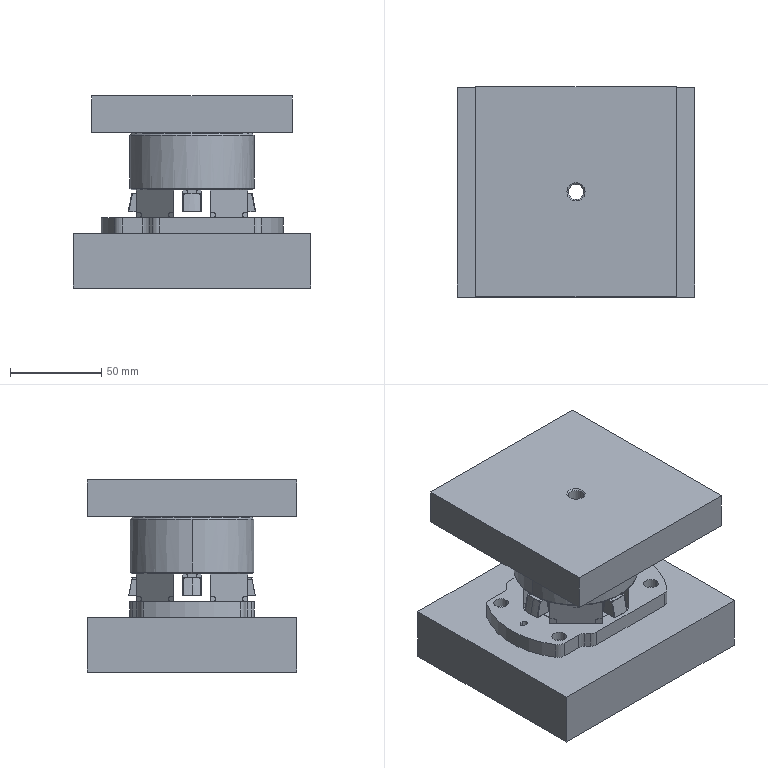NC program | NX | posted with a generic post | part box 130 x 115 x 105.2 mm
Lines 1665 to 1812 of 1812:
(122 , TOOL : ER25-D4-32_G)
N3298 T12 M6
N3300 G54
N3302 G17 G0 G90 X-1.197 Y34.94 B0. C0. S5000 M3
N3304 G43 Z50. H12
N3306 G94 G1 Z-10. F4500.
N3308 G41 X-1.2 Y34.74 F1000. D12
N3310 Y34.34
N3312 G3 X0. Y33.14 R1.2
N3314 G1 X2.68
N3316 G2 X6.681 Y30.511 R4.36
N3318 X6.863 Y30.01 R4.36 F917.
N3320 X6.982 Y29.491 R4.36 F833.
N3322 X7.036 Y28.96 R4.36 F750.
N3324 G1 X7.04 Y28.78 F667.
N3326 Y28.427
N3328 Y27.894 F583.
N3330 Y27.36 F500.
N3332 G2 X7.061 Y26.911 R2.06
N3334 G1 X7.063 Y26.829
N3336 G3 X7.398 Y26.455 R0.44 F667.
N3338 X7.762 Y26.53 R0.44 F833.
N3340 G1 X7.885 Y26.615
N3342 G2 X9.69 Y26.813 R2.06 F1000.
N3344 X9.69 Y-26.813 R28.51
N3346 X9.421 Y-26.89 R2.06
N3348 X8.891 Y-26.933 R2.06 F917.
N3350 X8.367 Y-26.839 R2.06 F833.
N3352 X7.885 Y-26.615 R2.06 F750.
N3354 G1 X7.762 Y-26.53 F667.
N3356 G3 X7.398 Y-26.455 R0.44
N3358 X7.063 Y-26.829 R0.44 F583.
N3360 G1 X7.061 Y-26.911 F500.
N3362 G2 X7.04 Y-27.36 R2.06
N3364 G1 Y-27.78
N3366 X7.039 Y-27.894
N3368 G2 X6.992 Y-28.425 R4.36 F667.
N3370 X6.881 Y-28.946 R4.36 F833.
N3372 X2.68 Y-32.14 R4.36 F1000.
N3374 G1 X-2.68
N3376 G2 X-6.183 Y-30.376 R4.36
N3378 X-6.474 Y-29.929 R4.36 F917.
N3380 X-6.708 Y-29.45 R4.36 F833.
N3382 X-6.881 Y-28.946 R4.36 F750.
N3384 X-6.992 Y-28.425 R4.36 F667.
N3386 X-7.039 Y-27.894 R4.36 F583.
N3388 G1 X-7.04 Y-27.78 F500.
N3390 Y-27.36
N3392 G2 X-7.061 Y-26.911 R2.06
N3394 G1 X-7.063 Y-26.829
N3396 G3 X-7.398 Y-26.455 R0.44 F667.
N3398 X-7.762 Y-26.53 R0.44 F833.
N3400 G1 X-7.885 Y-26.615
N3402 G2 X-9.69 Y-26.813 R2.06 F1000.
N3404 X-9.69 Y26.813 R28.51
N3406 X-9.421 Y26.89 R2.06
N3408 X-8.891 Y26.933 R2.06 F917.
N3410 X-8.367 Y26.839 R2.06 F833.
N3412 X-7.885 Y26.615 R2.06 F750.
N3414 G1 X-7.762 Y26.53 F667.
N3416 G3 X-7.398 Y26.455 R0.44
N3418 X-7.063 Y26.829 R0.44 F583.
N3420 G1 X-7.061 Y26.911 F500.
N3422 G2 X-7.04 Y27.36 R2.06
N3424 G1 Y27.894
N3426 Y28.427 F667.
N3428 Y28.78 F833.
N3430 X-7.036 Y28.96
N3432 G2 X-2.68 Y33.14 R4.36 F1000.
N3434 G1 X0.
N3436 X0.5
N3438 G3 X1.7 Y34.34 R1.2
N3440 G40
N3442 G1 X1.697 Y34.54
N3444 X-1.197 Y34.53
N3446 G41 X-1.2 Y34.33
N3448 G3 X0. Y33.13 R1.2
N3450 G1 X2.68
N3452 G2 X6.671 Y30.51 R4.35
N3454 X6.853 Y30.009 R4.35 F917.
N3456 X6.972 Y29.49 R4.35 F833.
N3458 X7.026 Y28.96 R4.35 F750.
N3460 G1 X7.03 Y28.78 F667.
N3462 Y28.426
N3464 Y27.893 F583.
N3466 Y27.36 F500.
N3468 G2 X7.051 Y26.912 R2.05
N3470 G1 X7.053 Y26.828
N3472 G3 X7.383 Y26.449 R0.45 F667.
N3474 X7.768 Y26.522 R0.45 F833.
N3476 G1 X7.873 Y26.595
N3478 G2 X9.686 Y26.803 R2.05 F1000.
N3480 X9.686 Y-26.803 R28.5
N3482 X9.406 Y-26.883 R2.05
N3484 X8.876 Y-26.922 R2.05 F917.
N3486 X8.353 Y-26.824 R2.05 F833.
N3488 X7.873 Y-26.595 R2.05 F750.
N3490 G1 X7.768 Y-26.522 F667.
N3492 G3 X7.383 Y-26.449 R0.45
N3494 X7.053 Y-26.828 R0.45 F583.
N3496 G1 X7.051 Y-26.912 F500.
N3498 G2 X7.03 Y-27.36 R2.05
N3500 G1 Y-27.78
N3502 X7.029 Y-27.893
N3504 G2 X6.982 Y-28.424 R4.35 F667.
N3506 X6.871 Y-28.945 R4.35 F833.
N3508 X2.68 Y-32.13 R4.35 F1000.
N3510 G1 X-2.68
N3512 G2 X-6.172 Y-30.374 R4.35
N3514 X-6.463 Y-29.928 R4.35 F917.
N3516 X-6.697 Y-29.449 R4.35 F833.
N3518 X-6.871 Y-28.945 R4.35 F750.
N3520 X-6.982 Y-28.424 R4.35 F667.
N3522 X-7.029 Y-27.893 R4.35 F583.
N3524 G1 X-7.03 Y-27.78 F500.
N3526 Y-27.36
N3528 G2 X-7.051 Y-26.912 R2.05
N3530 G1 X-7.053 Y-26.828
N3532 G3 X-7.383 Y-26.449 R0.45 F667.
N3534 X-7.768 Y-26.522 R0.45 F833.
N3536 G1 X-7.873 Y-26.595
N3538 G2 X-9.686 Y-26.803 R2.05 F1000.
N3540 X-9.686 Y26.803 R28.5
N3542 X-9.406 Y26.883 R2.05
N3544 X-8.876 Y26.922 R2.05 F917.
N3546 X-8.353 Y26.824 R2.05 F833.
N3548 X-7.873 Y26.595 R2.05 F750.
N3550 G1 X-7.768 Y26.522 F667.
N3552 G3 X-7.383 Y26.449 R0.45
N3554 X-7.053 Y26.828 R0.45 F583.
N3556 G1 X-7.051 Y26.912 F500.
N3558 G2 X-7.03 Y27.36 R2.05
N3560 G1 Y27.893
N3562 Y28.426 F667.
N3564 Y28.78 F833.
N3566 X-7.026 Y28.96
N3568 G2 X-2.68 Y33.13 R4.35 F1000.
N3570 G1 X0.
N3572 X0.5
N3574 G3 X1.7 Y34.33 R1.2
N3576 G1 Y34.74
N3578 G40
N3580 X1.697 Y34.94
N3582 G0 Z50.
N3584 M5
N3586 M2